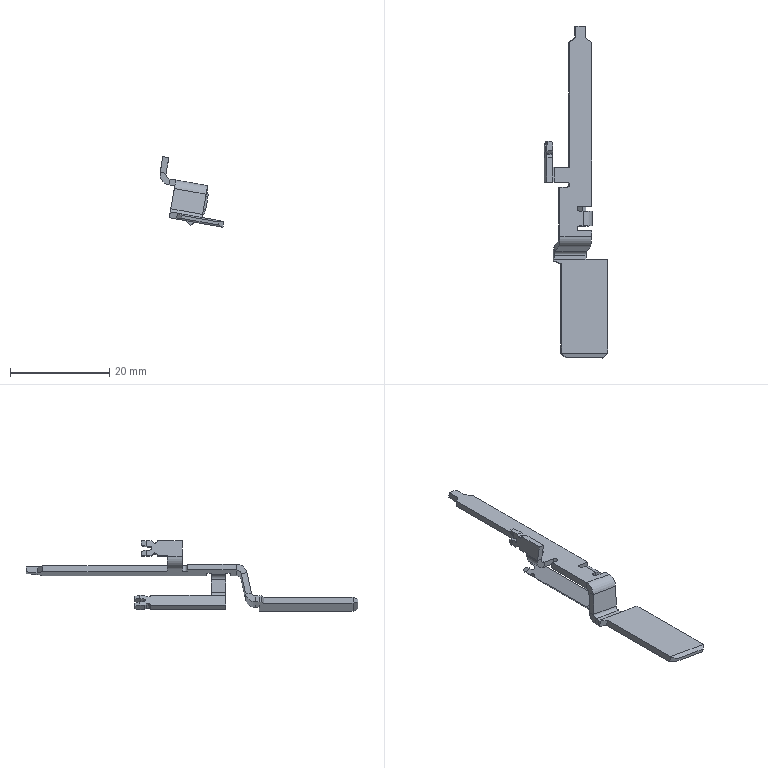Part | SolidWorks | features BaseBody 1 | 1 solid | 109 faces | box 12.902 x 66.9 x 14.209 mm | volume 657.962 mm3 | plane 88 | cylinder 21 | commonest cylinder face diameters 1 x9 2 x4 4.4 x4 0.8 x2 1.6 x1 4 x1